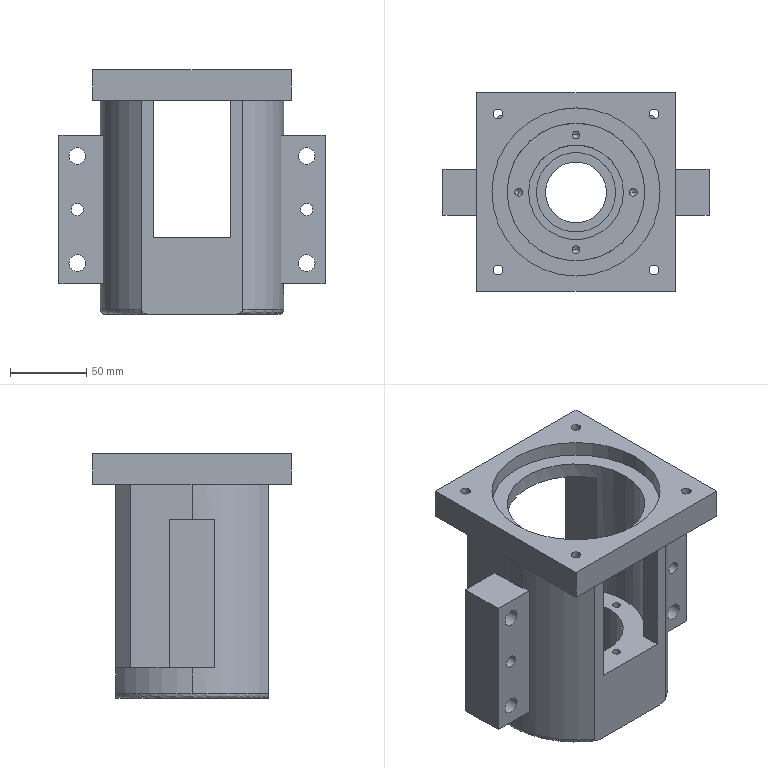Part | STEP file | 45L Z-Direction Motor Mount | 1 solid | 100 faces | box 174 x 130 x 160 mm | volume 1032339 mm3 | cylinder 51 | plane 38 | cone 8 | spline 3 | commonest cylinder face diameters 5 x8 6.5 x8 11 x8 17 x8 8 x4 52 x4